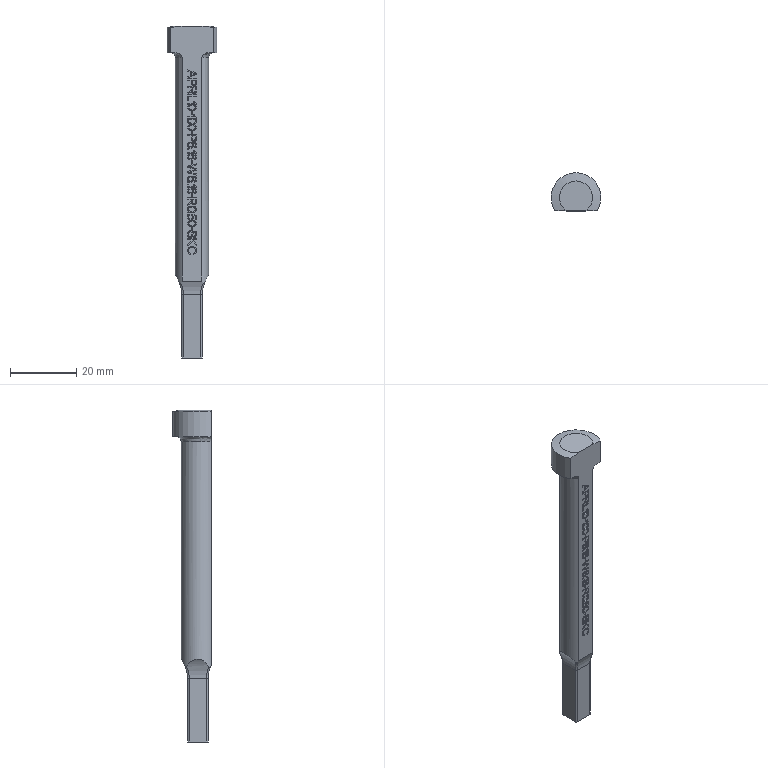Part | STEP file | PN_0053_id1726_x_t | 1 solid | 423 faces | box 15 x 11.5 x 100 mm | volume 7176 mm3 | plane 293 | cylinder 124 | spline 5 | cone 1 | commonest cylinder face diameters 1.141 x5 1.361 x5 1.365 x5 1.381 x5 1.816 x5 2.037 x5